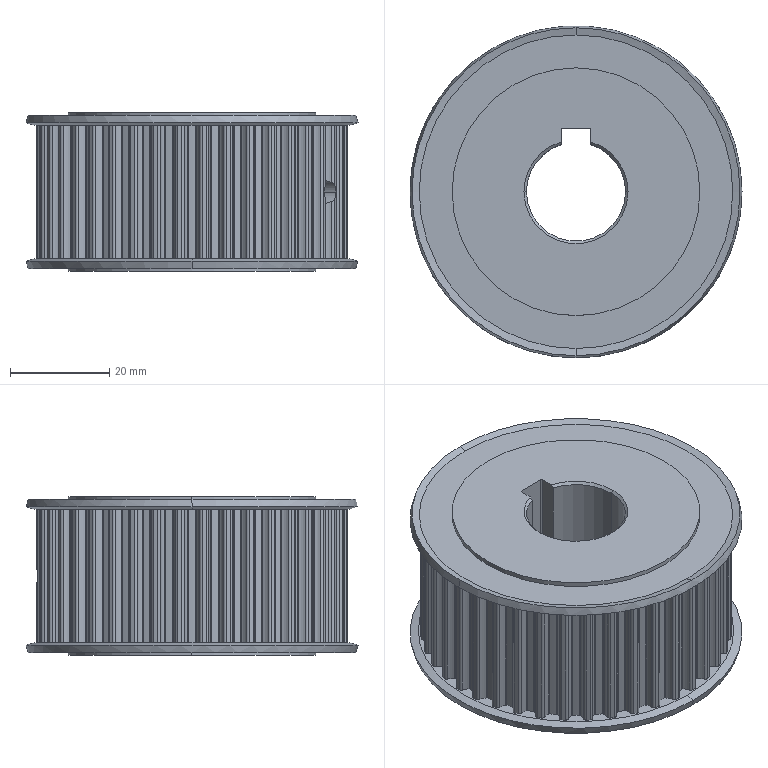Part | STEP file | EBJ52-S5M250-40-A-N-d20 | 1 solid | 412 faces | box 67 x 67 x 32 mm | volume 81650 mm3 | cylinder 385 | cone 18 | plane 9 | commonest cylinder face diameters 1.1 x103 0.5 x96 6.55 x90 59.16 x43 62.7 x40 4.917 x4